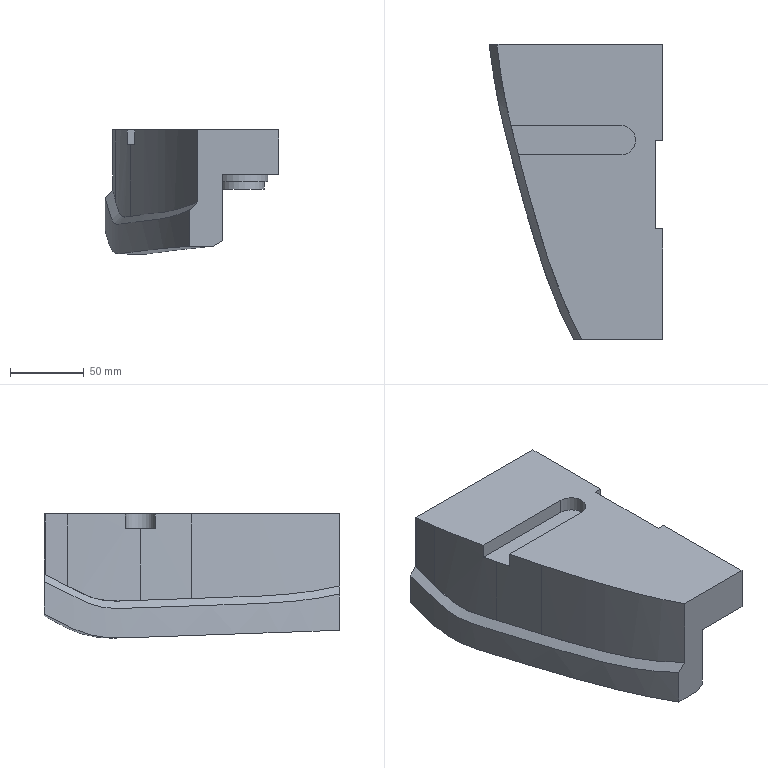Part | NX | features solid 2 | 1 solid | 37 faces | box 117.645 x 200 x 83.978 mm | volume 776577 mm3 | plane 18 | spline 13 | cylinder 6 | commonest cylinder face diameters 35 x3 30 x2 20 x1